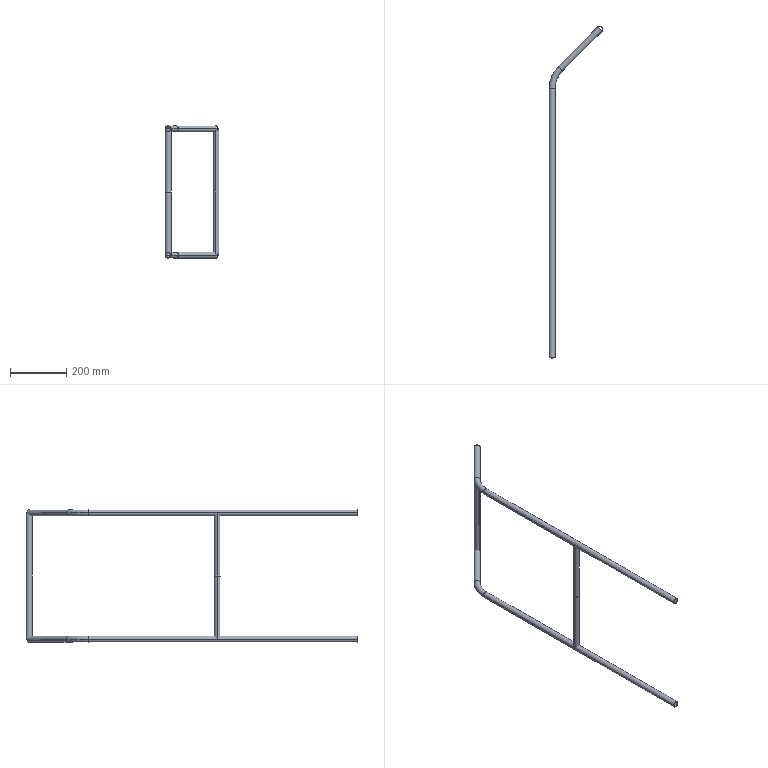Part | SolidWorks | features WeldMemberFeat 3, MirrorSolid 1, WeldmentFeature 1 | 9 solids | 54 faces | box 192.011 x 1181 x 471.3 mm | volume 463241 mm3 | cylinder 28 | plane 18 | torus 8 | commonest cylinder face diameters 16.7 x14 21.3 x14
STEP:
#1=CARTESIAN_POINT('',(-10.65,458.579,0.));
#2=VERTEX_POINT('',#1);
#3=CARTESIAN_POINT('',(10.65,458.579,0.));
#4=VERTEX_POINT('',#3);
#5=CARTESIAN_POINT('',(0.,458.579,0.));
#6=DIRECTION('',(0.,1.,0.));
#7=DIRECTION('',(-1.,0.,0.));
#8=AXIS2_PLACEMENT_3D('',#5,#6,#7);
#9=CIRCLE('',#8,10.65);
#10=EDGE_CURVE('',#2,#4,#9,.T.);
#11=ORIENTED_EDGE('',*,*,#10,.F.);
#12=CARTESIAN_POINT('',(-10.65,-500.,0.));
#13=VERTEX_POINT('',#12);
#14=CARTESIAN_POINT('',(-10.65,458.579,0.));
#15=DIRECTION('',(0.,-1.,0.));
#16=VECTOR('',#15,1000.);
#17=LINE('',#14,#16);
#18=EDGE_CURVE('',#2,#13,#17,.T.);
#19=ORIENTED_EDGE('',*,*,#18,.T.);
#20=CARTESIAN_POINT('',(10.65,-500.,0.));
#21=VERTEX_POINT('',#20);
#22=CARTESIAN_POINT('',(0.,-500.,0.));
#23=DIRECTION('',(0.,1.,0.));
#24=DIRECTION('',(-1.,0.,0.));
#25=AXIS2_PLACEMENT_3D('',#22,#23,#24);
#26=CIRCLE('',#25,10.65);
#27=EDGE_CURVE('',#13,#21,#26,.T.);
#28=ORIENTED_EDGE('',*,*,#27,.T.);
#29=CARTESIAN_POINT('',(10.65,458.579,0.));
#30=DIRECTION('',(0.,-1.,0.));
#31=VECTOR('',#30,1000.);
#32=LINE('',#29,#31);
#33=EDGE_CURVE('',#4,#21,#32,.T.);
#34=ORIENTED_EDGE('',*,*,#33,.F.);
#35=EDGE_LOOP('',(#11,#19,#28,#34));
#36=FACE_OUTER_BOUND('',#35,.T.);
#37=CARTESIAN_POINT('',(0.,458.579,0.));
#38=DIRECTION('',(0.,-1.,0.));
#39=DIRECTION('',(1.,0.,0.));
#40=AXIS2_PLACEMENT_3D('',#37,#38,#39);
#41=CYLINDRICAL_SURFACE('',#40,10.65);
#42=ADVANCED_FACE('',(#36),#41,.T.);
#43=CARTESIAN_POINT('',(8.35,458.579,0.));
#44=VERTEX_POINT('',#43);
#45=CARTESIAN_POINT('',(-8.35,458.579,0.));
#46=VERTEX_POINT('',#45);
#47=CARTESIAN_POINT('',(0.,458.579,0.));
#48=DIRECTION('',(0.,1.,0.));
#49=DIRECTION('',(-1.,0.,0.));
#50=AXIS2_PLACEMENT_3D('',#47,#48,#49);
#51=CIRCLE('',#50,8.35);
#52=EDGE_CURVE('',#44,#46,#51,.T.);
#53=ORIENTED_EDGE('',*,*,#52,.T.);
#54=CARTESIAN_POINT('',(-8.35,-500.,0.));
#55=VERTEX_POINT('',#54);
#56=CARTESIAN_POINT('',(-8.35,458.579,0.));
#57=DIRECTION('',(0.,-1.,0.));
#58=VECTOR('',#57,1000.);
#59=LINE('',#56,#58);
#60=EDGE_CURVE('',#46,#55,#59,.T.);
#61=ORIENTED_EDGE('',*,*,#60,.T.);
#62=CARTESIAN_POINT('',(8.35,-500.,0.));
#63=VERTEX_POINT('',#62);
#64=CARTESIAN_POINT('',(0.,-500.,0.));
#65=DIRECTION('',(0.,1.,0.));
#66=DIRECTION('',(-1.,0.,0.));
#67=AXIS2_PLACEMENT_3D('',#64,#65,#66);
#68=CIRCLE('',#67,8.35);
#69=EDGE_CURVE('',#63,#55,#68,.T.);
#70=ORIENTED_EDGE('',*,*,#69,.F.);
#71=CARTESIAN_POINT('',(8.35,458.579,0.));
#72=DIRECTION('',(0.,-1.,0.));
#73=VECTOR('',#72,1000.);
#74=LINE('',#71,#73);
#75=EDGE_CURVE('',#44,#63,#74,.T.);
#76=ORIENTED_EDGE('',*,*,#75,.F.);
#77=EDGE_LOOP('',(#53,#61,#70,#76));
#78=FACE_OUTER_BOUND('',#77,.T.);
#79=CARTESIAN_POINT('',(0.,458.579,0.));
#80=DIRECTION('',(0.,-1.,0.));
#81=DIRECTION('',(1.,0.,0.));
#82=AXIS2_PLACEMENT_3D('',#79,#80,#81);
#83=CYLINDRICAL_SURFACE('',#82,8.35);
#84=ADVANCED_FACE('',(#78),#83,.F.);
#85=ORIENTED_EDGE('',*,*,#60,.F.);
#86=CARTESIAN_POINT('',(0.,458.579,0.));
#87=DIRECTION('',(0.,1.,0.));
#88=DIRECTION('',(-1.,0.,0.));
#89=AXIS2_PLACEMENT_3D('',#86,#87,#88);
#90=CIRCLE('',#89,8.35);
#91=EDGE_CURVE('',#46,#44,#90,.T.);
#92=ORIENTED_EDGE('',*,*,#91,.T.);
#93=ORIENTED_EDGE('',*,*,#75,.T.);
#94=CARTESIAN_POINT('',(0.,-500.,0.));
#95=DIRECTION('',(0.,1.,0.));
#96=DIRECTION('',(-1.,0.,0.));
#97=AXIS2_PLACEMENT_3D('',#94,#95,#96);
#98=CIRCLE('',#97,8.35);
#99=EDGE_CURVE('',#55,#63,#98,.T.);
#100=ORIENTED_EDGE('',*,*,#99,.F.);
#101=EDGE_LOOP('',(#85,#92,#93,#100));
#102=FACE_OUTER_BOUND('',#101,.T.);
#103=CARTESIAN_POINT('',(0.,458.579,0.));
#104=DIRECTION('',(0.,-1.,0.));
#105=DIRECTION('',(1.,0.,0.));
#106=AXIS2_PLACEMENT_3D('',#103,#104,#105);
#107=CYLINDRICAL_SURFACE('',#106,8.35);
#108=ADVANCED_FACE('',(#102),#107,.F.);
#109=ORIENTED_EDGE('',*,*,#18,.F.);
#110=CARTESIAN_POINT('',(0.,458.579,0.));
#111=DIRECTION('',(0.,1.,0.));
#112=DIRECTION('',(-1.,0.,0.));
#113=AXIS2_PLACEMENT_3D('',#110,#111,#112);
#114=CIRCLE('',#113,10.65);
#115=EDGE_CURVE('',#4,#2,#114,.T.);
#116=ORIENTED_EDGE('',*,*,#115,.F.);
#117=ORIENTED_EDGE('',*,*,#33,.T.);
#118=CARTESIAN_POINT('',(0.,-500.,0.));
#119=DIRECTION('',(0.,1.,0.));
#120=DIRECTION('',(-1.,0.,0.));
#121=AXIS2_PLACEMENT_3D('',#118,#119,#120);
#122=CIRCLE('',#121,10.65);
#123=EDGE_CURVE('',#21,#13,#122,.T.);
#124=ORIENTED_EDGE('',*,*,#123,.T.);
#125=EDGE_LOOP('',(#109,#116,#117,#124));
#126=FACE_OUTER_BOUND('',#125,.T.);
#127=CARTESIAN_POINT('',(0.,458.579,0.));
#128=DIRECTION('',(0.,-1.,0.));
#129=DIRECTION('',(1.,0.,0.));
#130=AXIS2_PLACEMENT_3D('',#127,#128,#129);
#131=CYLINDRICAL_SURFACE('',#130,10.65);
#132=ADVANCED_FACE('',(#126),#131,.T.);
#133=ORIENTED_EDGE('',*,*,#69,.T.);
#134=ORIENTED_EDGE('',*,*,#99,.T.);
#135=EDGE_LOOP('',(#133,#134));
#136=FACE_BOUND('',#135,.T.);
#137=ORIENTED_EDGE('',*,*,#123,.F.);
#138=ORIENTED_EDGE('',*,*,#27,.F.);
#139=EDGE_LOOP('',(#137,#138));
#140=FACE_OUTER_BOUND('',#139,.T.);
#141=CARTESIAN_POINT('',(0.,-500.,0.));
#142=DIRECTION('',(0.,1.,0.));
#143=DIRECTION('',(-1.,0.,0.));
#144=AXIS2_PLACEMENT_3D('',#141,#142,#143);
#145=PLANE('',#144);
#146=ADVANCED_FACE('',(#136,#140),#145,.F.);
#147=ORIENTED_EDGE('',*,*,#52,.F.);
#148=ORIENTED_EDGE('',*,*,#91,.F.);
#149=EDGE_LOOP('',(#147,#148));
#150=FACE_BOUND('',#149,.T.);
#151=ORIENTED_EDGE('',*,*,#115,.T.);
#152=ORIENTED_EDGE('',*,*,#10,.T.);
#153=EDGE_LOOP('',(#151,#152));
#154=FACE_OUTER_BOUND('',#153,.T.);
#155=CARTESIAN_POINT('',(0.,458.579,0.));
#156=DIRECTION('',(0.,1.,0.));
#157=DIRECTION('',(-1.,0.,0.));
#158=AXIS2_PLACEMENT_3D('',#155,#156,#157);
#159=PLANE('',#158);
#160=ADVANCED_FACE('',(#150,#154),#159,.T.);
#161=CLOSED_SHELL('',(#42,#84,#108,#132,#146,#160));
#162=MANIFOLD_SOLID_BREP('',#161);
#163=CARTESIAN_POINT('',(21.759,536.82,0.));
#164=VERTEX_POINT('',#163);
#165=CARTESIAN_POINT('',(36.82,521.759,0.));
#166=VERTEX_POINT('',#165);
#167=CARTESIAN_POINT('',(29.289,529.289,0.));
#168=DIRECTION('',(0.7071,0.7071,0.));
#169=DIRECTION('',(-0.7071,0.7071,0.));
#170=AXIS2_PLACEMENT_3D('',#167,#168,#169);
#171=CIRCLE('',#170,10.65);
#172=EDGE_CURVE('',#164,#166,#171,.T.);
#173=ORIENTED_EDGE('',*,*,#172,.F.);
#174=CARTESIAN_POINT('',(-10.65,458.579,0.));
#175=VERTEX_POINT('',#174);
#176=CARTESIAN_POINT('',(100.,458.579,0.));
#177=DIRECTION('',(0.,0.,1.));
#178=DIRECTION('',(1.,0.,0.));
#179=AXIS2_PLACEMENT_3D('',#176,#177,#178);
#180=CIRCLE('',#179,110.65);
#181=EDGE_CURVE('',#164,#175,#180,.T.);
#182=ORIENTED_EDGE('',*,*,#181,.T.);
#183=CARTESIAN_POINT('',(10.65,458.579,0.));
#184=VERTEX_POINT('',#183);
#185=CARTESIAN_POINT('',(0.,458.579,0.));
#186=DIRECTION('',(0.,-1.,0.));
#187=DIRECTION('',(1.,0.,0.));
#188=AXIS2_PLACEMENT_3D('',#185,#186,#187);
#189=CIRCLE('',#188,10.65);
#190=EDGE_CURVE('',#184,#175,#189,.T.);
#191=ORIENTED_EDGE('',*,*,#190,.F.);
#192=CARTESIAN_POINT('',(100.,458.579,0.));
#193=DIRECTION('',(0.,0.,1.));
#194=DIRECTION('',(1.,0.,0.));
#195=AXIS2_PLACEMENT_3D('',#192,#193,#194);
#196=CIRCLE('',#195,89.35);
#197=EDGE_CURVE('',#166,#184,#196,.T.);
#198=ORIENTED_EDGE('',*,*,#197,.F.);
#199=EDGE_LOOP('',(#173,#182,#191,#198));
#200=FACE_OUTER_BOUND('',#199,.T.);
#201=CARTESIAN_POINT('',(100.,458.579,0.));
#202=DIRECTION('',(0.,0.,1.));
#203=DIRECTION('',(1.,0.,0.));
#204=AXIS2_PLACEMENT_3D('',#201,#202,#203);
#205=TOROIDAL_SURFACE('',#204,100.,10.65);
#206=ADVANCED_FACE('',(#200),#205,.T.);
#207=CARTESIAN_POINT('',(35.194,523.385,0.));
#208=VERTEX_POINT('',#207);
#209=CARTESIAN_POINT('',(23.385,535.194,0.));
#210=VERTEX_POINT('',#209);
#211=CARTESIAN_POINT('',(29.289,529.289,0.));
#212=DIRECTION('',(0.7071,0.7071,0.));
#213=DIRECTION('',(-0.7071,0.7071,0.));
#214=AXIS2_PLACEMENT_3D('',#211,#212,#213);
#215=CIRCLE('',#214,8.35);
#216=EDGE_CURVE('',#208,#210,#215,.T.);
#217=ORIENTED_EDGE('',*,*,#216,.T.);
#218=CARTESIAN_POINT('',(-8.35,458.579,0.));
#219=VERTEX_POINT('',#218);
#220=CARTESIAN_POINT('',(100.,458.579,0.));
#221=DIRECTION('',(0.,0.,1.));
#222=DIRECTION('',(1.,0.,0.));
#223=AXIS2_PLACEMENT_3D('',#220,#221,#222);
#224=CIRCLE('',#223,108.35);
#225=EDGE_CURVE('',#210,#219,#224,.T.);
#226=ORIENTED_EDGE('',*,*,#225,.T.);
#227=CARTESIAN_POINT('',(8.35,458.579,0.));
#228=VERTEX_POINT('',#227);
#229=CARTESIAN_POINT('',(0.,458.579,0.));
#230=DIRECTION('',(0.,-1.,0.));
#231=DIRECTION('',(1.,0.,0.));
#232=AXIS2_PLACEMENT_3D('',#229,#230,#231);
#233=CIRCLE('',#232,8.35);
#234=EDGE_CURVE('',#219,#228,#233,.T.);
#235=ORIENTED_EDGE('',*,*,#234,.T.);
#236=CARTESIAN_POINT('',(100.,458.579,0.));
#237=DIRECTION('',(0.,0.,1.));
#238=DIRECTION('',(1.,0.,0.));
#239=AXIS2_PLACEMENT_3D('',#236,#237,#238);
#240=CIRCLE('',#239,91.65);
#241=EDGE_CURVE('',#208,#228,#240,.T.);
#242=ORIENTED_EDGE('',*,*,#241,.F.);
#243=EDGE_LOOP('',(#217,#226,#235,#242));
#244=FACE_OUTER_BOUND('',#243,.T.);
#245=CARTESIAN_POINT('',(100.,458.579,0.));
#246=DIRECTION('',(0.,0.,1.));
#247=DIRECTION('',(1.,0.,0.));
#248=AXIS2_PLACEMENT_3D('',#245,#246,#247);
#249=TOROIDAL_SURFACE('',#248,100.,8.35);
#250=ADVANCED_FACE('',(#244),#249,.F.);
#251=ORIENTED_EDGE('',*,*,#225,.F.);
#252=CARTESIAN_POINT('',(29.289,529.289,0.));
#253=DIRECTION('',(0.7071,0.7071,0.));
#254=DIRECTION('',(-0.7071,0.7071,0.));
#255=AXIS2_PLACEMENT_3D('',#252,#253,#254);
#256=CIRCLE('',#255,8.35);
#257=EDGE_CURVE('',#210,#208,#256,.T.);
#258=ORIENTED_EDGE('',*,*,#257,.T.);
#259=ORIENTED_EDGE('',*,*,#241,.T.);
#260=CARTESIAN_POINT('',(0.,458.579,0.));
#261=DIRECTION('',(0.,-1.,0.));
#262=DIRECTION('',(1.,0.,0.));
#263=AXIS2_PLACEMENT_3D('',#260,#261,#262);
#264=CIRCLE('',#263,8.35);
#265=EDGE_CURVE('',#228,#219,#264,.T.);
#266=ORIENTED_EDGE('',*,*,#265,.T.);
#267=EDGE_LOOP('',(#251,#258,#259,#266));
#268=FACE_OUTER_BOUND('',#267,.T.);
#269=CARTESIAN_POINT('',(100.,458.579,0.));
#270=DIRECTION('',(0.,0.,1.));
#271=DIRECTION('',(1.,0.,0.));
#272=AXIS2_PLACEMENT_3D('',#269,#270,#271);
#273=TOROIDAL_SURFACE('',#272,100.,8.35);
#274=ADVANCED_FACE('',(#268),#273,.F.);
#275=ORIENTED_EDGE('',*,*,#181,.F.);
#276=CARTESIAN_POINT('',(29.289,529.289,0.));
#277=DIRECTION('',(0.7071,0.7071,0.));
#278=DIRECTION('',(-0.7071,0.7071,0.));
#279=AXIS2_PLACEMENT_3D('',#276,#277,#278);
#280=CIRCLE('',#279,10.65);
#281=EDGE_CURVE('',#166,#164,#280,.T.);
#282=ORIENTED_EDGE('',*,*,#281,.F.);
#283=ORIENTED_EDGE('',*,*,#197,.T.);
#284=CARTESIAN_POINT('',(0.,458.579,0.));
#285=DIRECTION('',(0.,-1.,0.));
#286=DIRECTION('',(1.,0.,0.));
#287=AXIS2_PLACEMENT_3D('',#284,#285,#286);
#288=CIRCLE('',#287,10.65);
#289=EDGE_CURVE('',#175,#184,#288,.T.);
#290=ORIENTED_EDGE('',*,*,#289,.F.);
#291=EDGE_LOOP('',(#275,#282,#283,#290));
#292=FACE_OUTER_BOUND('',#291,.T.);
#293=CARTESIAN_POINT('',(100.,458.579,0.));
#294=DIRECTION('',(0.,0.,1.));
#295=DIRECTION('',(1.,0.,0.));
#296=AXIS2_PLACEMENT_3D('',#293,#294,#295);
#297=TOROIDAL_SURFACE('',#296,100.,10.65);
#298=ADVANCED_FACE('',(#292),#297,.T.);
#299=ORIENTED_EDGE('',*,*,#216,.F.);
#300=ORIENTED_EDGE('',*,*,#257,.F.);
#301=EDGE_LOOP('',(#299,#300));
#302=FACE_BOUND('',#301,.T.);
#303=ORIENTED_EDGE('',*,*,#281,.T.);
#304=ORIENTED_EDGE('',*,*,#172,.T.);
#305=EDGE_LOOP('',(#303,#304));
#306=FACE_OUTER_BOUND('',#305,.T.);
#307=CARTESIAN_POINT('',(29.289,529.289,0.));
#308=DIRECTION('',(0.7071,0.7071,0.));
#309=DIRECTION('',(-0.7071,0.7071,0.));
#310=AXIS2_PLACEMENT_3D('',#307,#308,#309);
#311=PLANE('',#310);
#312=ADVANCED_FACE('',(#302,#306),#311,.T.);
#313=ORIENTED_EDGE('',*,*,#265,.F.);
#314=ORIENTED_EDGE('',*,*,#234,.F.);
#315=EDGE_LOOP('',(#313,#314));
#316=FACE_BOUND('',#315,.T.);
#317=ORIENTED_EDGE('',*,*,#190,.T.);
#318=ORIENTED_EDGE('',*,*,#289,.T.);
#319=EDGE_LOOP('',(#317,#318));
#320=FACE_OUTER_BOUND('',#319,.T.);
#321=CARTESIAN_POINT('',(0.,458.579,0.));
#322=DIRECTION('',(0.,-1.,0.));
#323=DIRECTION('',(1.,0.,0.));
#324=AXIS2_PLACEMENT_3D('',#321,#322,#323);
#325=PLANE('',#324);
#326=ADVANCED_FACE('',(#316,#320),#325,.T.);
#327=CLOSED_SHELL('',(#206,#250,#274,#298,#312,#326));
#328=MANIFOLD_SOLID_BREP('',#327);
#329=CARTESIAN_POINT('',(163.18,678.241,0.));
#330=VERTEX_POINT('',#329);
#331=CARTESIAN_POINT('',(178.241,663.18,0.));
#332=VERTEX_POINT('',#331);
#333=CARTESIAN_POINT('',(170.711,670.711,0.));
#334=DIRECTION('',(0.7071,0.7071,0.));
#335=DIRECTION('',(-0.7071,0.7071,0.));
#336=AXIS2_PLACEMENT_3D('',#333,#334,#335);
#337=CIRCLE('',#336,10.65);
#338=EDGE_CURVE('',#330,#332,#337,.T.);
#339=ORIENTED_EDGE('',*,*,#338,.F.);
#340=CARTESIAN_POINT('',(21.759,536.82,0.));
#341=VERTEX_POINT('',#340);
#342=CARTESIAN_POINT('',(163.18,678.241,0.));
#343=DIRECTION('',(-0.7071,-0.7071,0.));
#344=VECTOR('',#343,1000.);
#345=LINE('',#342,#344);
#346=EDGE_CURVE('',#330,#341,#345,.T.);
#347=ORIENTED_EDGE('',*,*,#346,.T.);
#348=CARTESIAN_POINT('',(36.82,521.759,0.));
#349=VERTEX_POINT('',#348);
#350=CARTESIAN_POINT('',(29.289,529.289,0.));
#351=DIRECTION('',(-0.7071,-0.7071,0.));
#352=DIRECTION('',(0.7071,-0.7071,0.));
#353=AXIS2_PLACEMENT_3D('',#350,#351,#352);
#354=CIRCLE('',#353,10.65);
#355=EDGE_CURVE('',#349,#341,#354,.T.);
#356=ORIENTED_EDGE('',*,*,#355,.F.);
#357=CARTESIAN_POINT('',(178.241,663.18,0.));
#358=DIRECTION('',(-0.7071,-0.7071,0.));
#359=VECTOR('',#358,1000.);
#360=LINE('',#357,#359);
#361=EDGE_CURVE('',#332,#349,#360,.T.);
#362=ORIENTED_EDGE('',*,*,#361,.F.);
#363=EDGE_LOOP('',(#339,#347,#356,#362));
#364=FACE_OUTER_BOUND('',#363,.T.);
#365=CARTESIAN_POINT('',(170.711,670.711,0.));
#366=DIRECTION('',(-0.7071,-0.7071,0.));
#367=DIRECTION('',(0.7071,-0.7071,0.));
#368=AXIS2_PLACEMENT_3D('',#365,#366,#367);
#369=CYLINDRICAL_SURFACE('',#368,10.65);
#370=ADVANCED_FACE('',(#364),#369,.T.);
#371=CARTESIAN_POINT('',(176.615,664.806,0.));
#372=VERTEX_POINT('',#371);
#373=CARTESIAN_POINT('',(164.806,676.615,0.));
#374=VERTEX_POINT('',#373);
#375=CARTESIAN_POINT('',(170.711,670.711,0.));
#376=DIRECTION('',(0.7071,0.7071,0.));
#377=DIRECTION('',(-0.7071,0.7071,0.));
#378=AXIS2_PLACEMENT_3D('',#375,#376,#377);
#379=CIRCLE('',#378,8.35);
#380=EDGE_CURVE('',#372,#374,#379,.T.);
#381=ORIENTED_EDGE('',*,*,#380,.T.);
#382=CARTESIAN_POINT('',(23.385,535.194,0.));
#383=VERTEX_POINT('',#382);
#384=CARTESIAN_POINT('',(164.806,676.615,0.));
#385=DIRECTION('',(-0.7071,-0.7071,0.));
#386=VECTOR('',#385,1000.);
#387=LINE('',#384,#386);
#388=EDGE_CURVE('',#374,#383,#387,.T.);
#389=ORIENTED_EDGE('',*,*,#388,.T.);
#390=CARTESIAN_POINT('',(35.194,523.385,0.));
#391=VERTEX_POINT('',#390);
#392=CARTESIAN_POINT('',(29.289,529.289,0.));
#393=DIRECTION('',(-0.7071,-0.7071,0.));
#394=DIRECTION('',(0.7071,-0.7071,0.));
#395=AXIS2_PLACEMENT_3D('',#392,#393,#394);
#396=CIRCLE('',#395,8.35);
#397=EDGE_CURVE('',#383,#391,#396,.T.);
#398=ORIENTED_EDGE('',*,*,#397,.T.);
#399=CARTESIAN_POINT('',(176.615,664.806,0.));
#400=DIRECTION('',(-0.7071,-0.7071,0.));
#401=VECTOR('',#400,1000.);
#402=LINE('',#399,#401);
#403=EDGE_CURVE('',#372,#391,#402,.T.);
#404=ORIENTED_EDGE('',*,*,#403,.F.);
#405=EDGE_LOOP('',(#381,#389,#398,#404));
#406=FACE_OUTER_BOUND('',#405,.T.);
#407=CARTESIAN_POINT('',(170.711,670.711,0.));
#408=DIRECTION('',(-0.7071,-0.7071,0.));
#409=DIRECTION('',(0.7071,-0.7071,0.));
#410=AXIS2_PLACEMENT_3D('',#407,#408,#409);
#411=CYLINDRICAL_SURFACE('',#410,8.35);
#412=ADVANCED_FACE('',(#406),#411,.F.);
#413=ORIENTED_EDGE('',*,*,#388,.F.);
#414=CARTESIAN_POINT('',(170.711,670.711,0.));
#415=DIRECTION('',(0.7071,0.7071,0.));
#416=DIRECTION('',(-0.7071,0.7071,0.));
#417=AXIS2_PLACEMENT_3D('',#414,#415,#416);
#418=CIRCLE('',#417,8.35);
#419=EDGE_CURVE('',#374,#372,#418,.T.);
#420=ORIENTED_EDGE('',*,*,#419,.T.);
#421=ORIENTED_EDGE('',*,*,#403,.T.);
#422=CARTESIAN_POINT('',(29.289,529.289,0.));
#423=DIRECTION('',(-0.7071,-0.7071,0.));
#424=DIRECTION('',(0.7071,-0.7071,0.));
#425=AXIS2_PLACEMENT_3D('',#422,#423,#424);
#426=CIRCLE('',#425,8.35);
#427=EDGE_CURVE('',#391,#383,#426,.T.);
#428=ORIENTED_EDGE('',*,*,#427,.T.);
#429=EDGE_LOOP('',(#413,#420,#421,#428));
#430=FACE_OUTER_BOUND('',#429,.T.);
#431=CARTESIAN_POINT('',(170.711,670.711,0.));
#432=DIRECTION('',(-0.7071,-0.7071,0.));
#433=DIRECTION('',(0.7071,-0.7071,0.));
#434=AXIS2_PLACEMENT_3D('',#431,#432,#433);
#435=CYLINDRICAL_SURFACE('',#434,8.35);
#436=ADVANCED_FACE('',(#430),#435,.F.);
#437=ORIENTED_EDGE('',*,*,#346,.F.);
#438=CARTESIAN_POINT('',(170.711,670.711,0.));
#439=DIRECTION('',(0.7071,0.7071,0.));
#440=DIRECTION('',(-0.7071,0.7071,0.));
#441=AXIS2_PLACEMENT_3D('',#438,#439,#440);
#442=CIRCLE('',#441,10.65);
#443=EDGE_CURVE('',#332,#330,#442,.T.);
#444=ORIENTED_EDGE('',*,*,#443,.F.);
#445=ORIENTED_EDGE('',*,*,#361,.T.);
#446=CARTESIAN_POINT('',(29.289,529.289,0.));
#447=DIRECTION('',(-0.7071,-0.7071,0.));
#448=DIRECTION('',(0.7071,-0.7071,0.));
#449=AXIS2_PLACEMENT_3D('',#446,#447,#448);
#450=CIRCLE('',#449,10.65);
#451=EDGE_CURVE('',#341,#349,#450,.T.);
#452=ORIENTED_EDGE('',*,*,#451,.F.);
#453=EDGE_LOOP('',(#437,#444,#445,#452));
#454=FACE_OUTER_BOUND('',#453,.T.);
#455=CARTESIAN_POINT('',(170.711,670.711,0.));
#456=DIRECTION('',(-0.7071,-0.7071,0.));
#457=DIRECTION('',(0.7071,-0.7071,0.));
#458=AXIS2_PLACEMENT_3D('',#455,#456,#457);
#459=CYLINDRICAL_SURFACE('',#458,10.65);
#460=ADVANCED_FACE('',(#454),#459,.T.);
#461=ORIENTED_EDGE('',*,*,#380,.F.);
#462=ORIENTED_EDGE('',*,*,#419,.F.);
#463=EDGE_LOOP('',(#461,#462));
#464=FACE_BOUND('',#463,.T.);
#465=ORIENTED_EDGE('',*,*,#443,.T.);
#466=ORIENTED_EDGE('',*,*,#338,.T.);
#467=EDGE_LOOP('',(#465,#466));
#468=FACE_OUTER_BOUND('',#467,.T.);
#469=CARTESIAN_POINT('',(170.711,670.711,0.));
#470=DIRECTION('',(0.7071,0.7071,0.));
#471=DIRECTION('',(-0.7071,0.7071,0.));
#472=AXIS2_PLACEMENT_3D('',#469,#470,#471);
#473=PLANE('',#472);
#474=ADVANCED_FACE('',(#464,#468),#473,.T.);
#475=ORIENTED_EDGE('',*,*,#427,.F.);
#476=ORIENTED_EDGE('',*,*,#397,.F.);
#477=EDGE_LOOP('',(#475,#476));
#478=FACE_BOUND('',#477,.T.);
#479=ORIENTED_EDGE('',*,*,#355,.T.);
#480=ORIENTED_EDGE('',*,*,#451,.T.);
#481=EDGE_LOOP('',(#479,#480));
#482=FACE_OUTER_BOUND('',#481,.T.);
#483=CARTESIAN_POINT('',(29.289,529.289,0.));
#484=DIRECTION('',(-0.7071,-0.7071,0.));
#485=DIRECTION('',(0.7071,-0.7071,0.));
#486=AXIS2_PLACEMENT_3D('',#483,#484,#485);
#487=PLANE('',#486);
#488=ADVANCED_FACE('',(#478,#482),#487,.T.);
#489=CLOSED_SHELL('',(#370,#412,#436,#460,#474,#488));
#490=MANIFOLD_SOLID_BREP('',#489);
#491=CARTESIAN_POINT('',(10.65,0.,225.));
#492=VERTEX_POINT('',#491);
#493=CARTESIAN_POINT('',(-10.65,0.,225.));
#494=VERTEX_POINT('',#493);
#495=CARTESIAN_POINT('',(0.,0.,225.));
#496=DIRECTION('',(0.,0.,1.));
#497=DIRECTION('',(1.,0.,0.));
#498=AXIS2_PLACEMENT_3D('',#495,#496,#497);
#499=CIRCLE('',#498,10.65);
#500=EDGE_CURVE('',#492,#494,#499,.T.);
#501=ORIENTED_EDGE('',*,*,#500,.F.);
#502=CARTESIAN_POINT('',(10.65,0.,0.));
#503=VERTEX_POINT('',#502);
#504=CARTESIAN_POINT('',(10.65,0.,225.));
#505=DIRECTION('',(0.,0.,-1.));
#506=VECTOR('',#505,1000.);
#507=LINE('',#504,#506);
#508=EDGE_CURVE('',#492,#503,#507,.T.);
#509=ORIENTED_EDGE('',*,*,#508,.T.);
#510=CARTESIAN_POINT('',(-10.65,0.,0.));
#511=VERTEX_POINT('',#510);
#512=CARTESIAN_POINT('',(0.,0.,0.));
#513=DIRECTION('',(0.,0.,1.));
#514=DIRECTION('',(1.,0.,0.));
#515=AXIS2_PLACEMENT_3D('',#512,#513,#514);
#516=CIRCLE('',#515,10.65);
#517=EDGE_CURVE('',#503,#511,#516,.T.);
#518=ORIENTED_EDGE('',*,*,#517,.T.);
#519=CARTESIAN_POINT('',(-10.65,0.,225.));
#520=DIRECTION('',(0.,0.,-1.));
#521=VECTOR('',#520,1000.);
#522=LINE('',#519,#521);
#523=EDGE_CURVE('',#494,#511,#522,.T.);
#524=ORIENTED_EDGE('',*,*,#523,.F.);
#525=EDGE_LOOP('',(#501,#509,#518,#524));
#526=FACE_OUTER_BOUND('',#525,.T.);
#527=CARTESIAN_POINT('',(0.,0.,225.));
#528=DIRECTION('',(0.,0.,-1.));
#529=DIRECTION('',(-1.,0.,0.));
#530=AXIS2_PLACEMENT_3D('',#527,#528,#529);
#531=CYLINDRICAL_SURFACE('',#530,10.65);
#532=ADVANCED_FACE('',(#526),#531,.T.);
#533=CARTESIAN_POINT('',(-8.35,0.,225.));
#534=VERTEX_POINT('',#533);
#535=CARTESIAN_POINT('',(8.35,0.,225.));
#536=VERTEX_POINT('',#535);
#537=CARTESIAN_POINT('',(0.,0.,225.));
#538=DIRECTION('',(0.,0.,1.));
#539=DIRECTION('',(1.,0.,0.));
#540=AXIS2_PLACEMENT_3D('',#537,#538,#539);
#541=CIRCLE('',#540,8.35);
#542=EDGE_CURVE('',#534,#536,#541,.T.);
#543=ORIENTED_EDGE('',*,*,#542,.T.);
#544=CARTESIAN_POINT('',(8.35,0.,0.));
#545=VERTEX_POINT('',#544);
#546=CARTESIAN_POINT('',(8.35,0.,225.));
#547=DIRECTION('',(0.,0.,-1.));
#548=VECTOR('',#547,1000.);
#549=LINE('',#546,#548);
#550=EDGE_CURVE('',#536,#545,#549,.T.);
#551=ORIENTED_EDGE('',*,*,#550,.T.);
#552=CARTESIAN_POINT('',(-8.35,0.,0.));
#553=VERTEX_POINT('',#552);
#554=CARTESIAN_POINT('',(0.,0.,0.));
#555=DIRECTION('',(0.,0.,1.));
#556=DIRECTION('',(1.,0.,0.));
#557=AXIS2_PLACEMENT_3D('',#554,#555,#556);
#558=CIRCLE('',#557,8.35);
#559=EDGE_CURVE('',#553,#545,#558,.T.);
#560=ORIENTED_EDGE('',*,*,#559,.F.);
#561=CARTESIAN_POINT('',(-8.35,0.,225.));
#562=DIRECTION('',(0.,0.,-1.));
#563=VECTOR('',#562,1000.);
#564=LINE('',#561,#563);
#565=EDGE_CURVE('',#534,#553,#564,.T.);
#566=ORIENTED_EDGE('',*,*,#565,.F.);
#567=EDGE_LOOP('',(#543,#551,#560,#566));
#568=FACE_OUTER_BOUND('',#567,.T.);
#569=CARTESIAN_POINT('',(0.,0.,225.));
#570=DIRECTION('',(0.,0.,-1.));
#571=DIRECTION('',(-1.,0.,0.));
#572=AXIS2_PLACEMENT_3D('',#569,#570,#571);
#573=CYLINDRICAL_SURFACE('',#572,8.35);
#574=ADVANCED_FACE('',(#568),#573,.F.);
#575=ORIENTED_EDGE('',*,*,#550,.F.);
#576=CARTESIAN_POINT('',(0.,0.,225.));
#577=DIRECTION('',(0.,0.,1.));
#578=DIRECTION('',(1.,0.,0.));
#579=AXIS2_PLACEMENT_3D('',#576,#577,#578);
#580=CIRCLE('',#579,8.35);
#581=EDGE_CURVE('',#536,#534,#580,.T.);
#582=ORIENTED_EDGE('',*,*,#581,.T.);
#583=ORIENTED_EDGE('',*,*,#565,.T.);
#584=CARTESIAN_POINT('',(0.,0.,0.));
#585=DIRECTION('',(0.,0.,1.));
#586=DIRECTION('',(1.,0.,0.));
#587=AXIS2_PLACEMENT_3D('',#584,#585,#586);
#588=CIRCLE('',#587,8.35);
#589=EDGE_CURVE('',#545,#553,#588,.T.);
#590=ORIENTED_EDGE('',*,*,#589,.F.);
#591=EDGE_LOOP('',(#575,#582,#583,#590));
#592=FACE_OUTER_BOUND('',#591,.T.);
#593=CARTESIAN_POINT('',(0.,0.,225.));
#594=DIRECTION('',(0.,0.,-1.));
#595=DIRECTION('',(-1.,0.,0.));
#596=AXIS2_PLACEMENT_3D('',#593,#594,#595);
#597=CYLINDRICAL_SURFACE('',#596,8.35);
#598=ADVANCED_FACE('',(#592),#597,.F.);
#599=ORIENTED_EDGE('',*,*,#508,.F.);
#600=CARTESIAN_POINT('',(0.,0.,225.));
#601=DIRECTION('',(0.,0.,1.));
#602=DIRECTION('',(1.,0.,0.));
#603=AXIS2_PLACEMENT_3D('',#600,#601,#602);
#604=CIRCLE('',#603,10.65);
#605=EDGE_CURVE('',#494,#492,#604,.T.);
#606=ORIENTED_EDGE('',*,*,#605,.F.);
#607=ORIENTED_EDGE('',*,*,#523,.T.);
#608=CARTESIAN_POINT('',(0.,0.,0.));
#609=DIRECTION('',(0.,0.,1.));
#610=DIRECTION('',(1.,0.,0.));
#611=AXIS2_PLACEMENT_3D('',#608,#609,#610);
#612=CIRCLE('',#611,10.65);
#613=EDGE_CURVE('',#511,#503,#612,.T.);
#614=ORIENTED_EDGE('',*,*,#613,.T.);
#615=EDGE_LOOP('',(#599,#606,#607,#614));
#616=FACE_OUTER_BOUND('',#615,.T.);
#617=CARTESIAN_POINT('',(0.,0.,225.));
#618=DIRECTION('',(0.,0.,-1.));
#619=DIRECTION('',(-1.,0.,0.));
#620=AXIS2_PLACEMENT_3D('',#617,#618,#619);
#621=CYLINDRICAL_SURFACE('',#620,10.65);
#622=ADVANCED_FACE('',(#616),#621,.T.);
#623=ORIENTED_EDGE('',*,*,#542,.F.);
#624=ORIENTED_EDGE('',*,*,#581,.F.);
#625=EDGE_LOOP('',(#623,#624));
#626=FACE_BOUND('',#625,.T.);
#627=ORIENTED_EDGE('',*,*,#605,.T.);
#628=ORIENTED_EDGE('',*,*,#500,.T.);
#629=EDGE_LOOP('',(#627,#628));
#630=FACE_OUTER_BOUND('',#629,.T.);
#631=CARTESIAN_POINT('',(0.,0.,225.));
#632=DIRECTION('',(0.,0.,1.));
#633=DIRECTION('',(1.,0.,0.));
#634=AXIS2_PLACEMENT_3D('',#631,#632,#633);
#635=PLANE('',#634);
#636=ADVANCED_FACE('',(#626,#630),#635,.T.);
#637=ORIENTED_EDGE('',*,*,#559,.T.);
#638=ORIENTED_EDGE('',*,*,#589,.T.);
#639=EDGE_LOOP('',(#637,#638));
#640=FACE_BOUND('',#639,.T.);
#641=ORIENTED_EDGE('',*,*,#613,.F.);
#642=ORIENTED_EDGE('',*,*,#517,.F.);
#643=EDGE_LOOP('',(#641,#642));
#644=FACE_OUTER_BOUND('',#643,.T.);
#645=CARTESIAN_POINT('',(0.,0.,0.));
#646=DIRECTION('',(0.,0.,1.));
#647=DIRECTION('',(1.,0.,0.));
#648=AXIS2_PLACEMENT_3D('',#645,#646,#647);
#649=PLANE('',#648);
#650=ADVANCED_FACE('',(#640,#644),#649,.F.);
#651=CLOSED_SHELL('',(#532,#574,#598,#622,#636,#650));
#652=MANIFOLD_SOLID_BREP('',#651);
#653=CARTESIAN_POINT('',(178.241,663.18,450.));
#654=VERTEX_POINT('',#653);
#655=CARTESIAN_POINT('',(163.18,678.241,450.));
#656=VERTEX_POINT('',#655);
#657=CARTESIAN_POINT('',(170.711,670.711,450.));
#658=DIRECTION('',(-0.7071,-0.7071,0.));
#659=DIRECTION('',(-0.7071,0.7071,0.));
#660=AXIS2_PLACEMENT_3D('',#657,#658,#659);
#661=CIRCLE('',#660,10.65);
#662=EDGE_CURVE('',#654,#656,#661,.T.);
#663=ORIENTED_EDGE('',*,*,#662,.T.);
#664=CARTESIAN_POINT('',(21.759,536.82,450.));
#665=VERTEX_POINT('',#664);
#666=CARTESIAN_POINT('',(163.18,678.241,450.));
#667=DIRECTION('',(-0.7071,-0.7071,0.));
#668=VECTOR('',#667,1000.);
#669=LINE('',#666,#668);
#670=EDGE_CURVE('',#656,#665,#669,.T.);
#671=ORIENTED_EDGE('',*,*,#670,.T.);
#672=CARTESIAN_POINT('',(36.82,521.759,450.));
#673=VERTEX_POINT('',#672);
#674=CARTESIAN_POINT('',(29.289,529.289,450.));
#675=DIRECTION('',(0.7071,0.7071,0.));
#676=DIRECTION('',(0.7071,-0.7071,0.));
#677=AXIS2_PLACEMENT_3D('',#674,#675,#676);
#678=CIRCLE('',#677,10.65);
#679=EDGE_CURVE('',#665,#673,#678,.T.);
#680=ORIENTED_EDGE('',*,*,#679,.T.);
#681=CARTESIAN_POINT('',(178.241,663.18,450.));
#682=DIRECTION('',(-0.7071,-0.7071,0.));
#683=VECTOR('',#682,1000.);
#684=LINE('',#681,#683);
#685=EDGE_CURVE('',#654,#673,#684,.T.);
#686=ORIENTED_EDGE('',*,*,#685,.F.);
#687=EDGE_LOOP('',(#663,#671,#680,#686));
#688=FACE_OUTER_BOUND('',#687,.T.);
#689=CARTESIAN_POINT('',(170.711,670.711,450.));
#690=DIRECTION('',(-0.7071,-0.7071,0.));
#691=DIRECTION('',(0.7071,-0.7071,0.));
#692=AXIS2_PLACEMENT_3D('',#689,#690,#691);
#693=CYLINDRICAL_SURFACE('',#692,10.65);
#694=ADVANCED_FACE('',(#688),#693,.T.);
#695=CARTESIAN_POINT('',(164.806,676.615,450.));
#696=VERTEX_POINT('',#695);
#697=CARTESIAN_POINT('',(176.615,664.806,450.));
#698=VERTEX_POINT('',#697);
#699=CARTESIAN_POINT('',(170.711,670.711,450.));
#700=DIRECTION('',(-0.7071,-0.7071,0.));
#701=DIRECTION('',(-0.7071,0.7071,0.));
#702=AXIS2_PLACEMENT_3D('',#699,#700,#701);
#703=CIRCLE('',#702,8.35);
#704=EDGE_CURVE('',#696,#698,#703,.T.);
#705=ORIENTED_EDGE('',*,*,#704,.F.);
#706=CARTESIAN_POINT('',(23.385,535.194,450.));
#707=VERTEX_POINT('',#706);
#708=CARTESIAN_POINT('',(164.806,676.615,450.));
#709=DIRECTION('',(-0.7071,-0.7071,0.));
#710=VECTOR('',#709,1000.);
#711=LINE('',#708,#710);
#712=EDGE_CURVE('',#696,#707,#711,.T.);
#713=ORIENTED_EDGE('',*,*,#712,.T.);
#714=CARTESIAN_POINT('',(35.194,523.385,450.));
#715=VERTEX_POINT('',#714);
#716=CARTESIAN_POINT('',(29.289,529.289,450.));
#717=DIRECTION('',(0.7071,0.7071,0.));
#718=DIRECTION('',(0.7071,-0.7071,0.));
#719=AXIS2_PLACEMENT_3D('',#716,#717,#718);
#720=CIRCLE('',#719,8.35);
#721=EDGE_CURVE('',#715,#707,#720,.T.);
#722=ORIENTED_EDGE('',*,*,#721,.F.);
#723=CARTESIAN_POINT('',(176.615,664.806,450.));
#724=DIRECTION('',(-0.7071,-0.7071,0.));
#725=VECTOR('',#724,1000.);
#726=LINE('',#723,#725);
#727=EDGE_CURVE('',#698,#715,#726,.T.);
#728=ORIENTED_EDGE('',*,*,#727,.F.);
#729=EDGE_LOOP('',(#705,#713,#722,#728));
#730=FACE_OUTER_BOUND('',#729,.T.);
#731=CARTESIAN_POINT('',(170.711,670.711,450.));
#732=DIRECTION('',(-0.7071,-0.7071,0.));
#733=DIRECTION('',(0.7071,-0.7071,0.));
#734=AXIS2_PLACEMENT_3D('',#731,#732,#733);
#735=CYLINDRICAL_SURFACE('',#734,8.35);
#736=ADVANCED_FACE('',(#730),#735,.F.);
#737=ORIENTED_EDGE('',*,*,#712,.F.);
#738=CARTESIAN_POINT('',(170.711,670.711,450.));
#739=DIRECTION('',(-0.7071,-0.7071,0.));
#740=DIRECTION('',(-0.7071,0.7071,0.));
#741=AXIS2_PLACEMENT_3D('',#738,#739,#740);
#742=CIRCLE('',#741,8.35);
#743=EDGE_CURVE('',#698,#696,#742,.T.);
#744=ORIENTED_EDGE('',*,*,#743,.F.);
#745=ORIENTED_EDGE('',*,*,#727,.T.);
#746=CARTESIAN_POINT('',(29.289,529.289,450.));
#747=DIRECTION('',(0.7071,0.7071,0.));
#748=DIRECTION('',(0.7071,-0.7071,0.));
#749=AXIS2_PLACEMENT_3D('',#746,#747,#748);
#750=CIRCLE('',#749,8.35);
#751=EDGE_CURVE('',#707,#715,#750,.T.);
#752=ORIENTED_EDGE('',*,*,#751,.F.);
#753=EDGE_LOOP('',(#737,#744,#745,#752));
#754=FACE_OUTER_BOUND('',#753,.T.);
#755=CARTESIAN_POINT('',(170.711,670.711,450.));
#756=DIRECTION('',(-0.7071,-0.7071,0.));
#757=DIRECTION('',(0.7071,-0.7071,0.));
#758=AXIS2_PLACEMENT_3D('',#755,#756,#757);
#759=CYLINDRICAL_SURFACE('',#758,8.35);
#760=ADVANCED_FACE('',(#754),#759,.F.);
#761=ORIENTED_EDGE('',*,*,#670,.F.);
#762=CARTESIAN_POINT('',(170.711,670.711,450.));
#763=DIRECTION('',(-0.7071,-0.7071,0.));
#764=DIRECTION('',(-0.7071,0.7071,0.));
#765=AXIS2_PLACEMENT_3D('',#762,#763,#764);
#766=CIRCLE('',#765,10.65);
#767=EDGE_CURVE('',#656,#654,#766,.T.);
#768=ORIENTED_EDGE('',*,*,#767,.T.);
#769=ORIENTED_EDGE('',*,*,#685,.T.);
#770=CARTESIAN_POINT('',(29.289,529.289,450.));
#771=DIRECTION('',(0.7071,0.7071,0.));
#772=DIRECTION('',(0.7071,-0.7071,0.));
#773=AXIS2_PLACEMENT_3D('',#770,#771,#772);
#774=CIRCLE('',#773,10.65);
#775=EDGE_CURVE('',#673,#665,#774,.T.);
#776=ORIENTED_EDGE('',*,*,#775,.T.);
#777=EDGE_LOOP('',(#761,#768,#769,#776));
#778=FACE_OUTER_BOUND('',#777,.T.);
#779=CARTESIAN_POINT('',(170.711,670.711,450.));
#780=DIRECTION('',(-0.7071,-0.7071,0.));
#781=DIRECTION('',(0.7071,-0.7071,0.));
#782=AXIS2_PLACEMENT_3D('',#779,#780,#781);
#783=CYLINDRICAL_SURFACE('',#782,10.65);
#784=ADVANCED_FACE('',(#778),#783,.T.);
#785=ORIENTED_EDGE('',*,*,#743,.T.);
#786=ORIENTED_EDGE('',*,*,#704,.T.);
#787=EDGE_LOOP('',(#785,#786));
#788=FACE_BOUND('',#787,.T.);
#789=ORIENTED_EDGE('',*,*,#662,.F.);
#790=ORIENTED_EDGE('',*,*,#767,.F.);
#791=EDGE_LOOP('',(#789,#790));
#792=FACE_OUTER_BOUND('',#791,.T.);
#793=CARTESIAN_POINT('',(170.711,670.711,450.));
#794=DIRECTION('',(0.7071,0.7071,0.));
#795=DIRECTION('',(-0.7071,0.7071,0.));
#796=AXIS2_PLACEMENT_3D('',#793,#794,#795);
#797=PLANE('',#796);
#798=ADVANCED_FACE('',(#788,#792),#797,.T.);
#799=ORIENTED_EDGE('',*,*,#721,.T.);
#800=ORIENTED_EDGE('',*,*,#751,.T.);
#801=EDGE_LOOP('',(#799,#800));
#802=FACE_BOUND('',#801,.T.);
#803=ORIENTED_EDGE('',*,*,#775,.F.);
#804=ORIENTED_EDGE('',*,*,#679,.F.);
#805=EDGE_LOOP('',(#803,#804));
#806=FACE_OUTER_BOUND('',#805,.T.);
#807=CARTESIAN_POINT('',(29.289,529.289,450.));
#808=DIRECTION('',(-0.7071,-0.7071,0.));
#809=DIRECTION('',(0.7071,-0.7071,0.));
#810=AXIS2_PLACEMENT_3D('',#807,#808,#809);
#811=PLANE('',#810);
#812=ADVANCED_FACE('',(#802,#806),#811,.T.);
#813=CLOSED_SHELL('',(#694,#736,#760,#784,#798,#812));
#814=MANIFOLD_SOLID_BREP('',#813);
#815=CARTESIAN_POINT('',(10.65,458.579,450.));
#816=VERTEX_POINT('',#815);
#817=CARTESIAN_POINT('',(-10.65,458.579,450.));
#818=VERTEX_POINT('',#817);
#819=CARTESIAN_POINT('',(0.,458.579,450.));
#820=DIRECTION('',(0.,1.,0.));
#821=DIRECTION('',(1.,0.,0.));
#822=AXIS2_PLACEMENT_3D('',#819,#820,#821);
#823=CIRCLE('',#822,10.65);
#824=EDGE_CURVE('',#816,#818,#823,.T.);
#825=ORIENTED_EDGE('',*,*,#824,.T.);
#826=CARTESIAN_POINT('',(21.759,536.82,450.));
#827=VERTEX_POINT('',#826);
#828=CARTESIAN_POINT('',(100.,458.579,450.));
#829=DIRECTION('',(0.,0.,-1.));
#830=DIRECTION('',(-1.,0.,0.));
#831=AXIS2_PLACEMENT_3D('',#828,#829,#830);
#832=CIRCLE('',#831,110.65);
#833=EDGE_CURVE('',#818,#827,#832,.T.);
#834=ORIENTED_EDGE('',*,*,#833,.T.);
#835=CARTESIAN_POINT('',(36.82,521.759,450.));
#836=VERTEX_POINT('',#835);
#837=CARTESIAN_POINT('',(29.289,529.289,450.));
#838=DIRECTION('',(-0.7071,-0.7071,0.));
#839=DIRECTION('',(-0.7071,0.7071,0.));
#840=AXIS2_PLACEMENT_3D('',#837,#838,#839);
#841=CIRCLE('',#840,10.65);
#842=EDGE_CURVE('',#827,#836,#841,.T.);
#843=ORIENTED_EDGE('',*,*,#842,.T.);
#844=CARTESIAN_POINT('',(100.,458.579,450.));
#845=DIRECTION('',(0.,0.,-1.));
#846=DIRECTION('',(-1.,0.,0.));
#847=AXIS2_PLACEMENT_3D('',#844,#845,#846);
#848=CIRCLE('',#847,89.35);
#849=EDGE_CURVE('',#816,#836,#848,.T.);
#850=ORIENTED_EDGE('',*,*,#849,.F.);
#851=EDGE_LOOP('',(#825,#834,#843,#850));
#852=FACE_OUTER_BOUND('',#851,.T.);
#853=CARTESIAN_POINT('',(100.,458.579,450.));
#854=DIRECTION('',(0.,0.,-1.));
#855=DIRECTION('',(1.,0.,0.));
#856=AXIS2_PLACEMENT_3D('',#853,#854,#855);
#857=TOROIDAL_SURFACE('',#856,100.,10.65);
#858=ADVANCED_FACE('',(#852),#857,.T.);
#859=CARTESIAN_POINT('',(-8.35,458.579,450.));
#860=VERTEX_POINT('',#859);
#861=CARTESIAN_POINT('',(8.35,458.579,450.));
#862=VERTEX_POINT('',#861);
#863=CARTESIAN_POINT('',(0.,458.579,450.));
#864=DIRECTION('',(0.,1.,0.));
#865=DIRECTION('',(1.,0.,0.));
#866=AXIS2_PLACEMENT_3D('',#863,#864,#865);
#867=CIRCLE('',#866,8.35);
#868=EDGE_CURVE('',#860,#862,#867,.T.);
#869=ORIENTED_EDGE('',*,*,#868,.F.);
#870=CARTESIAN_POINT('',(23.385,535.194,450.));
#871=VERTEX_POINT('',#870);
#872=CARTESIAN_POINT('',(100.,458.579,450.));
#873=DIRECTION('',(0.,0.,-1.));
#874=DIRECTION('',(-1.,0.,0.));
#875=AXIS2_PLACEMENT_3D('',#872,#873,#874);
#876=CIRCLE('',#875,108.35);
#877=EDGE_CURVE('',#860,#871,#876,.T.);
#878=ORIENTED_EDGE('',*,*,#877,.T.);
#879=CARTESIAN_POINT('',(35.194,523.385,450.));
#880=VERTEX_POINT('',#879);
#881=CARTESIAN_POINT('',(29.289,529.289,450.));
#882=DIRECTION('',(-0.7071,-0.7071,0.));
#883=DIRECTION('',(-0.7071,0.7071,0.));
#884=AXIS2_PLACEMENT_3D('',#881,#882,#883);
#885=CIRCLE('',#884,8.35);
#886=EDGE_CURVE('',#880,#871,#885,.T.);
#887=ORIENTED_EDGE('',*,*,#886,.F.);
#888=CARTESIAN_POINT('',(100.,458.579,450.));
#889=DIRECTION('',(0.,0.,-1.));
#890=DIRECTION('',(-1.,0.,0.));
#891=AXIS2_PLACEMENT_3D('',#888,#889,#890);
#892=CIRCLE('',#891,91.65);
#893=EDGE_CURVE('',#862,#880,#892,.T.);
#894=ORIENTED_EDGE('',*,*,#893,.F.);
#895=EDGE_LOOP('',(#869,#878,#887,#894));
#896=FACE_OUTER_BOUND('',#895,.T.);
#897=CARTESIAN_POINT('',(100.,458.579,450.));
#898=DIRECTION('',(0.,0.,-1.));
#899=DIRECTION('',(1.,0.,0.));
#900=AXIS2_PLACEMENT_3D('',#897,#898,#899);
#901=TOROIDAL_SURFACE('',#900,100.,8.35);
#902=ADVANCED_FACE('',(#896),#901,.F.);
#903=ORIENTED_EDGE('',*,*,#877,.F.);
#904=CARTESIAN_POINT('',(0.,458.579,450.));
#905=DIRECTION('',(0.,1.,0.));
#906=DIRECTION('',(1.,0.,0.));
#907=AXIS2_PLACEMENT_3D('',#904,#905,#906);
#908=CIRCLE('',#907,8.35);
#909=EDGE_CURVE('',#862,#860,#908,.T.);
#910=ORIENTED_EDGE('',*,*,#909,.F.);
#911=ORIENTED_EDGE('',*,*,#893,.T.);
#912=CARTESIAN_POINT('',(29.289,529.289,450.));
#913=DIRECTION('',(-0.7071,-0.7071,0.));
#914=DIRECTION('',(-0.7071,0.7071,0.));
#915=AXIS2_PLACEMENT_3D('',#912,#913,#914);
#916=CIRCLE('',#915,8.35);
#917=EDGE_CURVE('',#871,#880,#916,.T.);
#918=ORIENTED_EDGE('',*,*,#917,.F.);
#919=EDGE_LOOP('',(#903,#910,#911,#918));
#920=FACE_OUTER_BOUND('',#919,.T.);
#921=CARTESIAN_POINT('',(100.,458.579,450.));
#922=DIRECTION('',(0.,0.,-1.));
#923=DIRECTION('',(1.,0.,0.));
#924=AXIS2_PLACEMENT_3D('',#921,#922,#923);
#925=TOROIDAL_SURFACE('',#924,100.,8.35);
#926=ADVANCED_FACE('',(#920),#925,.F.);
#927=ORIENTED_EDGE('',*,*,#833,.F.);
#928=CARTESIAN_POINT('',(0.,458.579,450.));
#929=DIRECTION('',(0.,1.,0.));
#930=DIRECTION('',(1.,0.,0.));
#931=AXIS2_PLACEMENT_3D('',#928,#929,#930);
#932=CIRCLE('',#931,10.65);
#933=EDGE_CURVE('',#818,#816,#932,.T.);
#934=ORIENTED_EDGE('',*,*,#933,.T.);
#935=ORIENTED_EDGE('',*,*,#849,.T.);
#936=CARTESIAN_POINT('',(29.289,529.289,450.));
#937=DIRECTION('',(-0.7071,-0.7071,0.));
#938=DIRECTION('',(-0.7071,0.7071,0.));
#939=AXIS2_PLACEMENT_3D('',#936,#937,#938);
#940=CIRCLE('',#939,10.65);
#941=EDGE_CURVE('',#836,#827,#940,.T.);
#942=ORIENTED_EDGE('',*,*,#941,.T.);
#943=EDGE_LOOP('',(#927,#934,#935,#942));
#944=FACE_OUTER_BOUND('',#943,.T.);
#945=CARTESIAN_POINT('',(100.,458.579,450.));
#946=DIRECTION('',(0.,0.,-1.));
#947=DIRECTION('',(1.,0.,0.));
#948=AXIS2_PLACEMENT_3D('',#945,#946,#947);
#949=TOROIDAL_SURFACE('',#948,100.,10.65);
#950=ADVANCED_FACE('',(#944),#949,.T.);
#951=ORIENTED_EDGE('',*,*,#886,.T.);
#952=ORIENTED_EDGE('',*,*,#917,.T.);
#953=EDGE_LOOP('',(#951,#952));
#954=FACE_BOUND('',#953,.T.);
#955=ORIENTED_EDGE('',*,*,#941,.F.);
#956=ORIENTED_EDGE('',*,*,#842,.F.);
#957=EDGE_LOOP('',(#955,#956));
#958=FACE_OUTER_BOUND('',#957,.T.);
#959=CARTESIAN_POINT('',(29.289,529.289,450.));
#960=DIRECTION('',(0.7071,0.7071,0.));
#961=DIRECTION('',(-0.7071,0.7071,0.));
#962=AXIS2_PLACEMENT_3D('',#959,#960,#961);
#963=PLANE('',#962);
#964=ADVANCED_FACE('',(#954,#958),#963,.T.);
#965=ORIENTED_EDGE('',*,*,#909,.T.);
#966=ORIENTED_EDGE('',*,*,#868,.T.);
#967=EDGE_LOOP('',(#965,#966));
#968=FACE_BOUND('',#967,.T.);
#969=ORIENTED_EDGE('',*,*,#824,.F.);
#970=ORIENTED_EDGE('',*,*,#933,.F.);
#971=EDGE_LOOP('',(#969,#970));
#972=FACE_OUTER_BOUND('',#971,.T.);
#973=CARTESIAN_POINT('',(0.,458.579,450.));
#974=DIRECTION('',(0.,-1.,0.));
#975=DIRECTION('',(1.,0.,0.));
#976=AXIS2_PLACEMENT_3D('',#973,#974,#975);
#977=PLANE('',#976);
#978=ADVANCED_FACE('',(#968,#972),#977,.T.);
#979=CLOSED_SHELL('',(#858,#902,#926,#950,#964,#978));
#980=MANIFOLD_SOLID_BREP('',#979);
#981=CARTESIAN_POINT('',(10.65,458.579,450.));
#982=VERTEX_POINT('',#981);
#983=CARTESIAN_POINT('',(-10.65,458.579,450.));
#984=VERTEX_POINT('',#983);
#985=CARTESIAN_POINT('',(0.,458.579,450.));
#986=DIRECTION('',(0.,-1.,0.));
#987=DIRECTION('',(-1.,0.,0.));
#988=AXIS2_PLACEMENT_3D('',#985,#986,#987);
#989=CIRCLE('',#988,10.65);
#990=EDGE_CURVE('',#982,#984,#989,.T.);
#991=ORIENTED_EDGE('',*,*,#990,.T.);
#992=CARTESIAN_POINT('',(-10.65,-500.,450.));
#993=VERTEX_POINT('',#992);
#994=CARTESIAN_POINT('',(-10.65,458.579,450.));
#995=DIRECTION('',(0.,-1.,0.));
#996=VECTOR('',#995,1000.);
#997=LINE('',#994,#996);
#998=EDGE_CURVE('',#984,#993,#997,.T.);
#999=ORIENTED_EDGE('',*,*,#998,.T.);
#1000=CARTESIAN_POINT('',(10.65,-500.,450.));
#1001=VERTEX_POINT('',#1000);
#1002=CARTESIAN_POINT('',(0.,-500.,450.));
#1003=DIRECTION('',(0.,-1.,0.));
#1004=DIRECTION('',(-1.,0.,0.));
#1005=AXIS2_PLACEMENT_3D('',#1002,#1003,#1004);
#1006=CIRCLE('',#1005,10.65);
#1007=EDGE_CURVE('',#1001,#993,#1006,.T.);
#1008=ORIENTED_EDGE('',*,*,#1007,.F.);
#1009=CARTESIAN_POINT('',(10.65,458.579,450.));
#1010=DIRECTION('',(0.,-1.,0.));
#1011=VECTOR('',#1010,1000.);
#1012=LINE('',#1009,#1011);
#1013=EDGE_CURVE('',#982,#1001,#1012,.T.);
#1014=ORIENTED_EDGE('',*,*,#1013,.F.);
#1015=EDGE_LOOP('',(#991,#999,#1008,#1014));
#1016=FACE_OUTER_BOUND('',#1015,.T.);
#1017=CARTESIAN_POINT('',(0.,458.579,450.));
#1018=DIRECTION('',(0.,-1.,0.));
#1019=DIRECTION('',(1.,0.,0.));
#1020=AXIS2_PLACEMENT_3D('',#1017,#1018,#1019);
#1021=CYLINDRICAL_SURFACE('',#1020,10.65);
#1022=ADVANCED_FACE('',(#1016),#1021,.T.);
#1023=CARTESIAN_POINT('',(-8.35,458.579,450.));
#1024=VERTEX_POINT('',#1023);
#1025=CARTESIAN_POINT('',(8.35,458.579,450.));
#1026=VERTEX_POINT('',#1025);
#1027=CARTESIAN_POINT('',(0.,458.579,450.));
#1028=DIRECTION('',(0.,-1.,0.));
#1029=DIRECTION('',(-1.,0.,0.));
#1030=AXIS2_PLACEMENT_3D('',#1027,#1028,#1029);
#1031=CIRCLE('',#1030,8.35);
#1032=EDGE_CURVE('',#1024,#1026,#1031,.T.);
#1033=ORIENTED_EDGE('',*,*,#1032,.F.);
#1034=CARTESIAN_POINT('',(-8.35,-500.,450.));
#1035=VERTEX_POINT('',#1034);
#1036=CARTESIAN_POINT('',(-8.35,458.579,450.));
#1037=DIRECTION('',(0.,-1.,0.));
#1038=VECTOR('',#1037,1000.);
#1039=LINE('',#1036,#1038);
#1040=EDGE_CURVE('',#1024,#1035,#1039,.T.);
#1041=ORIENTED_EDGE('',*,*,#1040,.T.);
#1042=CARTESIAN_POINT('',(8.35,-500.,450.));
#1043=VERTEX_POINT('',#1042);
#1044=CARTESIAN_POINT('',(0.,-500.,450.));
#1045=DIRECTION('',(0.,-1.,0.));
#1046=DIRECTION('',(-1.,0.,0.));
#1047=AXIS2_PLACEMENT_3D('',#1044,#1045,#1046);
#1048=CIRCLE('',#1047,8.35);
#1049=EDGE_CURVE('',#1035,#1043,#1048,.T.);
#1050=ORIENTED_EDGE('',*,*,#1049,.T.);
#1051=CARTESIAN_POINT('',(8.35,458.579,450.));
#1052=DIRECTION('',(0.,-1.,0.));
#1053=VECTOR('',#1052,1000.);
#1054=LINE('',#1051,#1053);
#1055=EDGE_CURVE('',#1026,#1043,#1054,.T.);
#1056=ORIENTED_EDGE('',*,*,#1055,.F.);
#1057=EDGE_LOOP('',(#1033,#1041,#1050,#1056));
#1058=FACE_OUTER_BOUND('',#1057,.T.);
#1059=CARTESIAN_POINT('',(0.,458.579,450.));
#1060=DIRECTION('',(0.,-1.,0.));
#1061=DIRECTION('',(1.,0.,0.));
#1062=AXIS2_PLACEMENT_3D('',#1059,#1060,#1061);
#1063=CYLINDRICAL_SURFACE('',#1062,8.35);
#1064=ADVANCED_FACE('',(#1058),#1063,.F.);
#1065=ORIENTED_EDGE('',*,*,#1040,.F.);
#1066=CARTESIAN_POINT('',(0.,458.579,450.));
#1067=DIRECTION('',(0.,-1.,0.));
#1068=DIRECTION('',(-1.,0.,0.));
#1069=AXIS2_PLACEMENT_3D('',#1066,#1067,#1068);
#1070=CIRCLE('',#1069,8.35);
#1071=EDGE_CURVE('',#1026,#1024,#1070,.T.);
#1072=ORIENTED_EDGE('',*,*,#1071,.F.);
#1073=ORIENTED_EDGE('',*,*,#1055,.T.);
#1074=CARTESIAN_POINT('',(0.,-500.,450.));
#1075=DIRECTION('',(0.,-1.,0.));
#1076=DIRECTION('',(-1.,0.,0.));
#1077=AXIS2_PLACEMENT_3D('',#1074,#1075,#1076);
#1078=CIRCLE('',#1077,8.35);
#1079=EDGE_CURVE('',#1043,#1035,#1078,.T.);
#1080=ORIENTED_EDGE('',*,*,#1079,.T.);
#1081=EDGE_LOOP('',(#1065,#1072,#1073,#1080));
#1082=FACE_OUTER_BOUND('',#1081,.T.);
#1083=CARTESIAN_POINT('',(0.,458.579,450.));
#1084=DIRECTION('',(0.,-1.,0.));
#1085=DIRECTION('',(1.,0.,0.));
#1086=AXIS2_PLACEMENT_3D('',#1083,#1084,#1085);
#1087=CYLINDRICAL_SURFACE('',#1086,8.35);
#1088=ADVANCED_FACE('',(#1082),#1087,.F.);
#1089=ORIENTED_EDGE('',*,*,#998,.F.);
#1090=CARTESIAN_POINT('',(0.,458.579,450.));
#1091=DIRECTION('',(0.,-1.,0.));
#1092=DIRECTION('',(-1.,0.,0.));
#1093=AXIS2_PLACEMENT_3D('',#1090,#1091,#1092);
#1094=CIRCLE('',#1093,10.65);
#1095=EDGE_CURVE('',#984,#982,#1094,.T.);
#1096=ORIENTED_EDGE('',*,*,#1095,.T.);
#1097=ORIENTED_EDGE('',*,*,#1013,.T.);
#1098=CARTESIAN_POINT('',(0.,-500.,450.));
#1099=DIRECTION('',(0.,-1.,0.));
#1100=DIRECTION('',(-1.,0.,0.));
#1101=AXIS2_PLACEMENT_3D('',#1098,#1099,#1100);
#1102=CIRCLE('',#1101,10.65);
#1103=EDGE_CURVE('',#993,#1001,#1102,.T.);
#1104=ORIENTED_EDGE('',*,*,#1103,.F.);
#1105=EDGE_LOOP('',(#1089,#1096,#1097,#1104));
#1106=FACE_OUTER_BOUND('',#1105,.T.);
#1107=CARTESIAN_POINT('',(0.,458.579,450.));
#1108=DIRECTION('',(0.,-1.,0.));
#1109=DIRECTION('',(1.,0.,0.));
#1110=AXIS2_PLACEMENT_3D('',#1107,#1108,#1109);
#1111=CYLINDRICAL_SURFACE('',#1110,10.65);
#1112=ADVANCED_FACE('',(#1106),#1111,.T.);
#1113=ORIENTED_EDGE('',*,*,#1079,.F.);
#1114=ORIENTED_EDGE('',*,*,#1049,.F.);
#1115=EDGE_LOOP('',(#1113,#1114));
#1116=FACE_BOUND('',#1115,.T.);
#1117=ORIENTED_EDGE('',*,*,#1007,.T.);
#1118=ORIENTED_EDGE('',*,*,#1103,.T.);
#1119=EDGE_LOOP('',(#1117,#1118));
#1120=FACE_OUTER_BOUND('',#1119,.T.);
#1121=CARTESIAN_POINT('',(0.,-500.,450.));
#1122=DIRECTION('',(0.,1.,0.));
#1123=DIRECTION('',(-1.,0.,0.));
#1124=AXIS2_PLACEMENT_3D('',#1121,#1122,#1123);
#1125=PLANE('',#1124);
#1126=ADVANCED_FACE('',(#1116,#1120),#1125,.F.);
#1127=ORIENTED_EDGE('',*,*,#1071,.T.);
#1128=ORIENTED_EDGE('',*,*,#1032,.T.);
#1129=EDGE_LOOP('',(#1127,#1128));
#1130=FACE_BOUND('',#1129,.T.);
#1131=ORIENTED_EDGE('',*,*,#990,.F.);
#1132=ORIENTED_EDGE('',*,*,#1095,.F.);
#1133=EDGE_LOOP('',(#1131,#1132));
#1134=FACE_OUTER_BOUND('',#1133,.T.);
#1135=CARTESIAN_POINT('',(0.,458.579,450.));
#1136=DIRECTION('',(0.,1.,0.));
#1137=DIRECTION('',(-1.,0.,0.));
#1138=AXIS2_PLACEMENT_3D('',#1135,#1136,#1137);
#1139=PLANE('',#1138);
#1140=ADVANCED_FACE('',(#1130,#1134),#1139,.T.);
#1141=CLOSED_SHELL('',(#1022,#1064,#1088,#1112,#1126,#1140));
#1142=MANIFOLD_SOLID_BREP('',#1141);
#1143=CARTESIAN_POINT('',(-10.65,0.,225.));
#1144=VERTEX_POINT('',#1143);
#1145=CARTESIAN_POINT('',(10.65,0.,225.));
#1146=VERTEX_POINT('',#1145);
#1147=CARTESIAN_POINT('',(0.,0.,225.));
#1148=DIRECTION('',(0.,0.,1.));
#1149=DIRECTION('',(1.,0.,0.));
#1150=AXIS2_PLACEMENT_3D('',#1147,#1148,#1149);
#1151=CIRCLE('',#1150,10.65);
#1152=EDGE_CURVE('',#1144,#1146,#1151,.T.);
#1153=ORIENTED_EDGE('',*,*,#1152,.T.);
#1154=CARTESIAN_POINT('',(10.65,0.,450.));
#1155=VERTEX_POINT('',#1154);
#1156=CARTESIAN_POINT('',(10.65,0.,225.));
#1157=DIRECTION('',(0.,0.,1.));
#1158=VECTOR('',#1157,1000.);
#1159=LINE('',#1156,#1158);
#1160=EDGE_CURVE('',#1146,#1155,#1159,.T.);
#1161=ORIENTED_EDGE('',*,*,#1160,.T.);
#1162=CARTESIAN_POINT('',(-10.65,0.,450.));
#1163=VERTEX_POINT('',#1162);
#1164=CARTESIAN_POINT('',(0.,0.,450.));
#1165=DIRECTION('',(0.,0.,1.));
#1166=DIRECTION('',(1.,0.,0.));
#1167=AXIS2_PLACEMENT_3D('',#1164,#1165,#1166);
#1168=CIRCLE('',#1167,10.65);
#1169=EDGE_CURVE('',#1163,#1155,#1168,.T.);
#1170=ORIENTED_EDGE('',*,*,#1169,.F.);
#1171=CARTESIAN_POINT('',(-10.65,0.,225.));
#1172=DIRECTION('',(0.,0.,1.));
#1173=VECTOR('',#1172,1000.);
#1174=LINE('',#1171,#1173);
#1175=EDGE_CURVE('',#1144,#1163,#1174,.T.);
#1176=ORIENTED_EDGE('',*,*,#1175,.F.);
#1177=EDGE_LOOP('',(#1153,#1161,#1170,#1176));
#1178=FACE_OUTER_BOUND('',#1177,.T.);
#1179=CARTESIAN_POINT('',(0.,0.,225.));
#1180=DIRECTION('',(0.,0.,1.));
#1181=DIRECTION('',(-1.,0.,0.));
#1182=AXIS2_PLACEMENT_3D('',#1179,#1180,#1181);
#1183=CYLINDRICAL_SURFACE('',#1182,10.65);
#1184=ADVANCED_FACE('',(#1178),#1183,.T.);
#1185=CARTESIAN_POINT('',(8.35,0.,225.));
#1186=VERTEX_POINT('',#1185);
#1187=CARTESIAN_POINT('',(-8.35,0.,225.));
#1188=VERTEX_POINT('',#1187);
#1189=CARTESIAN_POINT('',(0.,0.,225.));
#1190=DIRECTION('',(0.,0.,1.));
#1191=DIRECTION('',(1.,0.,0.));
#1192=AXIS2_PLACEMENT_3D('',#1189,#1190,#1191);
#1193=CIRCLE('',#1192,8.35);
#1194=EDGE_CURVE('',#1186,#1188,#1193,.T.);
#1195=ORIENTED_EDGE('',*,*,#1194,.F.);
#1196=CARTESIAN_POINT('',(8.35,0.,450.));
#1197=VERTEX_POINT('',#1196);
#1198=CARTESIAN_POINT('',(8.35,0.,225.));
#1199=DIRECTION('',(0.,0.,1.));
#1200=VECTOR('',#1199,1000.);
#1201=LINE('',#1198,#1200);
#1202=EDGE_CURVE('',#1186,#1197,#1201,.T.);
#1203=ORIENTED_EDGE('',*,*,#1202,.T.);
#1204=CARTESIAN_POINT('',(-8.35,0.,450.));
#1205=VERTEX_POINT('',#1204);
#1206=CARTESIAN_POINT('',(0.,0.,450.));
#1207=DIRECTION('',(0.,0.,1.));
#1208=DIRECTION('',(1.,0.,0.));
#1209=AXIS2_PLACEMENT_3D('',#1206,#1207,#1208);
#1210=CIRCLE('',#1209,8.35);
#1211=EDGE_CURVE('',#1197,#1205,#1210,.T.);
#1212=ORIENTED_EDGE('',*,*,#1211,.T.);
#1213=CARTESIAN_POINT('',(-8.35,0.,225.));
#1214=DIRECTION('',(0.,0.,1.));
#1215=VECTOR('',#1214,1000.);
#1216=LINE('',#1213,#1215);
#1217=EDGE_CURVE('',#1188,#1205,#1216,.T.);
#1218=ORIENTED_EDGE('',*,*,#1217,.F.);
#1219=EDGE_LOOP('',(#1195,#1203,#1212,#1218));
#1220=FACE_OUTER_BOUND('',#1219,.T.);
#1221=CARTESIAN_POINT('',(0.,0.,225.));
#1222=DIRECTION('',(0.,0.,1.));
#1223=DIRECTION('',(-1.,0.,0.));
#1224=AXIS2_PLACEMENT_3D('',#1221,#1222,#1223);
#1225=CYLINDRICAL_SURFACE('',#1224,8.35);
#1226=ADVANCED_FACE('',(#1220),#1225,.F.);
#1227=ORIENTED_EDGE('',*,*,#1202,.F.);
#1228=CARTESIAN_POINT('',(0.,0.,225.));
#1229=DIRECTION('',(0.,0.,1.));
#1230=DIRECTION('',(1.,0.,0.));
#1231=AXIS2_PLACEMENT_3D('',#1228,#1229,#1230);
#1232=CIRCLE('',#1231,8.35);
#1233=EDGE_CURVE('',#1188,#1186,#1232,.T.);
#1234=ORIENTED_EDGE('',*,*,#1233,.F.);
#1235=ORIENTED_EDGE('',*,*,#1217,.T.);
#1236=CARTESIAN_POINT('',(0.,0.,450.));
#1237=DIRECTION('',(0.,0.,1.));
#1238=DIRECTION('',(1.,0.,0.));
#1239=AXIS2_PLACEMENT_3D('',#1236,#1237,#1238);
#1240=CIRCLE('',#1239,8.35);
#1241=EDGE_CURVE('',#1205,#1197,#1240,.T.);
#1242=ORIENTED_EDGE('',*,*,#1241,.T.);
#1243=EDGE_LOOP('',(#1227,#1234,#1235,#1242));
#1244=FACE_OUTER_BOUND('',#1243,.T.);
#1245=CARTESIAN_POINT('',(0.,0.,225.));
#1246=DIRECTION('',(0.,0.,1.));
#1247=DIRECTION('',(-1.,0.,0.));
#1248=AXIS2_PLACEMENT_3D('',#1245,#1246,#1247);
#1249=CYLINDRICAL_SURFACE('',#1248,8.35);
#1250=ADVANCED_FACE('',(#1244),#1249,.F.);
#1251=ORIENTED_EDGE('',*,*,#1160,.F.);
#1252=CARTESIAN_POINT('',(0.,0.,225.));
#1253=DIRECTION('',(0.,0.,1.));
#1254=DIRECTION('',(1.,0.,0.));
#1255=AXIS2_PLACEMENT_3D('',#1252,#1253,#1254);
#1256=CIRCLE('',#1255,10.65);
#1257=EDGE_CURVE('',#1146,#1144,#1256,.T.);
#1258=ORIENTED_EDGE('',*,*,#1257,.T.);
#1259=ORIENTED_EDGE('',*,*,#1175,.T.);
#1260=CARTESIAN_POINT('',(0.,0.,450.));
#1261=DIRECTION('',(0.,0.,1.));
#1262=DIRECTION('',(1.,0.,0.));
#1263=AXIS2_PLACEMENT_3D('',#1260,#1261,#1262);
#1264=CIRCLE('',#1263,10.65);
#1265=EDGE_CURVE('',#1155,#1163,#1264,.T.);
#1266=ORIENTED_EDGE('',*,*,#1265,.F.);
#1267=EDGE_LOOP('',(#1251,#1258,#1259,#1266));
#1268=FACE_OUTER_BOUND('',#1267,.T.);
#1269=CARTESIAN_POINT('',(0.,0.,225.));
#1270=DIRECTION('',(0.,0.,1.));
#1271=DIRECTION('',(-1.,0.,0.));
#1272=AXIS2_PLACEMENT_3D('',#1269,#1270,#1271);
#1273=CYLINDRICAL_SURFACE('',#1272,10.65);
#1274=ADVANCED_FACE('',(#1268),#1273,.T.);
#1275=ORIENTED_EDGE('',*,*,#1233,.T.);
#1276=ORIENTED_EDGE('',*,*,#1194,.T.);
#1277=EDGE_LOOP('',(#1275,#1276));
#1278=FACE_BOUND('',#1277,.T.);
#1279=ORIENTED_EDGE('',*,*,#1152,.F.);
#1280=ORIENTED_EDGE('',*,*,#1257,.F.);
#1281=EDGE_LOOP('',(#1279,#1280));
#1282=FACE_OUTER_BOUND('',#1281,.T.);
#1283=CARTESIAN_POINT('',(0.,0.,225.));
#1284=DIRECTION('',(0.,0.,-1.));
#1285=DIRECTION('',(1.,0.,0.));
#1286=AXIS2_PLACEMENT_3D('',#1283,#1284,#1285);
#1287=PLANE('',#1286);
#1288=ADVANCED_FACE('',(#1278,#1282),#1287,.T.);
#1289=ORIENTED_EDGE('',*,*,#1241,.F.);
#1290=ORIENTED_EDGE('',*,*,#1211,.F.);
#1291=EDGE_LOOP('',(#1289,#1290));
#1292=FACE_BOUND('',#1291,.T.);
#1293=ORIENTED_EDGE('',*,*,#1169,.T.);
#1294=ORIENTED_EDGE('',*,*,#1265,.T.);
#1295=EDGE_LOOP('',(#1293,#1294));
#1296=FACE_OUTER_BOUND('',#1295,.T.);
#1297=CARTESIAN_POINT('',(0.,0.,450.));
#1298=DIRECTION('',(0.,0.,-1.));
#1299=DIRECTION('',(1.,0.,0.));
#1300=AXIS2_PLACEMENT_3D('',#1297,#1298,#1299);
#1301=PLANE('',#1300);
#1302=ADVANCED_FACE('',(#1292,#1296),#1301,.F.);
#1303=CLOSED_SHELL('',(#1184,#1226,#1250,#1274,#1288,#1302));
#1304=MANIFOLD_SOLID_BREP('',#1303);
#1305=CARTESIAN_POINT('',(170.711,681.361,0.));
#1306=VERTEX_POINT('',#1305);
#1307=CARTESIAN_POINT('',(170.711,660.061,0.));
#1308=VERTEX_POINT('',#1307);
#1309=CARTESIAN_POINT('',(170.711,670.711,0.));
#1310=DIRECTION('',(0.,0.,-1.));
#1311=DIRECTION('',(0.,1.,0.));
#1312=AXIS2_PLACEMENT_3D('',#1309,#1310,#1311);
#1313=CIRCLE('',#1312,10.65);
#1314=EDGE_CURVE('',#1306,#1308,#1313,.T.);
#1315=ORIENTED_EDGE('',*,*,#1314,.F.);
#1316=CARTESIAN_POINT('',(170.711,681.361,450.));
#1317=VERTEX_POINT('',#1316);
#1318=CARTESIAN_POINT('',(170.711,681.361,0.));
#1319=DIRECTION('',(0.,0.,1.));
#1320=VECTOR('',#1319,1000.);
#1321=LINE('',#1318,#1320);
#1322=EDGE_CURVE('',#1306,#1317,#1321,.T.);
#1323=ORIENTED_EDGE('',*,*,#1322,.T.);
#1324=CARTESIAN_POINT('',(170.711,660.061,450.));
#1325=VERTEX_POINT('',#1324);
#1326=CARTESIAN_POINT('',(170.711,670.711,450.));
#1327=DIRECTION('',(0.,0.,-1.));
#1328=DIRECTION('',(0.,1.,0.));
#1329=AXIS2_PLACEMENT_3D('',#1326,#1327,#1328);
#1330=CIRCLE('',#1329,10.65);
#1331=EDGE_CURVE('',#1317,#1325,#1330,.T.);
#1332=ORIENTED_EDGE('',*,*,#1331,.T.);
#1333=CARTESIAN_POINT('',(170.711,660.061,0.));
#1334=DIRECTION('',(0.,0.,1.));
#1335=VECTOR('',#1334,1000.);
#1336=LINE('',#1333,#1335);
#1337=EDGE_CURVE('',#1308,#1325,#1336,.T.);
#1338=ORIENTED_EDGE('',*,*,#1337,.F.);
#1339=EDGE_LOOP('',(#1315,#1323,#1332,#1338));
#1340=FACE_OUTER_BOUND('',#1339,.T.);
#1341=CARTESIAN_POINT('',(170.711,670.711,0.));
#1342=DIRECTION('',(0.,0.,1.));
#1343=DIRECTION('',(0.,-1.,0.));
#1344=AXIS2_PLACEMENT_3D('',#1341,#1342,#1343);
#1345=CYLINDRICAL_SURFACE('',#1344,10.65);
#1346=ADVANCED_FACE('',(#1340),#1345,.T.);
#1347=CARTESIAN_POINT('',(170.711,662.361,0.));
#1348=VERTEX_POINT('',#1347);
#1349=CARTESIAN_POINT('',(170.711,679.061,0.));
#1350=VERTEX_POINT('',#1349);
#1351=CARTESIAN_POINT('',(170.711,670.711,0.));
#1352=DIRECTION('',(0.,0.,-1.));
#1353=DIRECTION('',(0.,1.,0.));
#1354=AXIS2_PLACEMENT_3D('',#1351,#1352,#1353);
#1355=CIRCLE('',#1354,8.35);
#1356=EDGE_CURVE('',#1348,#1350,#1355,.T.);
#1357=ORIENTED_EDGE('',*,*,#1356,.T.);
#1358=CARTESIAN_POINT('',(170.711,679.061,450.));
#1359=VERTEX_POINT('',#1358);
#1360=CARTESIAN_POINT('',(170.711,679.061,0.));
#1361=DIRECTION('',(0.,0.,1.));
#1362=VECTOR('',#1361,1000.);
#1363=LINE('',#1360,#1362);
#1364=EDGE_CURVE('',#1350,#1359,#1363,.T.);
#1365=ORIENTED_EDGE('',*,*,#1364,.T.);
#1366=CARTESIAN_POINT('',(170.711,662.361,450.));
#1367=VERTEX_POINT('',#1366);
#1368=CARTESIAN_POINT('',(170.711,670.711,450.));
#1369=DIRECTION('',(0.,0.,-1.));
#1370=DIRECTION('',(0.,1.,0.));
#1371=AXIS2_PLACEMENT_3D('',#1368,#1369,#1370);
#1372=CIRCLE('',#1371,8.35);
#1373=EDGE_CURVE('',#1367,#1359,#1372,.T.);
#1374=ORIENTED_EDGE('',*,*,#1373,.F.);
#1375=CARTESIAN_POINT('',(170.711,662.361,0.));
#1376=DIRECTION('',(0.,0.,1.));
#1377=VECTOR('',#1376,1000.);
#1378=LINE('',#1375,#1377);
#1379=EDGE_CURVE('',#1348,#1367,#1378,.T.);
#1380=ORIENTED_EDGE('',*,*,#1379,.F.);
#1381=EDGE_LOOP('',(#1357,#1365,#1374,#1380));
#1382=FACE_OUTER_BOUND('',#1381,.T.);
#1383=CARTESIAN_POINT('',(170.711,670.711,0.));
#1384=DIRECTION('',(0.,0.,1.));
#1385=DIRECTION('',(0.,-1.,0.));
#1386=AXIS2_PLACEMENT_3D('',#1383,#1384,#1385);
#1387=CYLINDRICAL_SURFACE('',#1386,8.35);
#1388=ADVANCED_FACE('',(#1382),#1387,.F.);
#1389=ORIENTED_EDGE('',*,*,#1364,.F.);
#1390=CARTESIAN_POINT('',(170.711,670.711,0.));
#1391=DIRECTION('',(0.,0.,-1.));
#1392=DIRECTION('',(0.,1.,0.));
#1393=AXIS2_PLACEMENT_3D('',#1390,#1391,#1392);
#1394=CIRCLE('',#1393,8.35);
#1395=EDGE_CURVE('',#1350,#1348,#1394,.T.);
#1396=ORIENTED_EDGE('',*,*,#1395,.T.);
#1397=ORIENTED_EDGE('',*,*,#1379,.T.);
#1398=CARTESIAN_POINT('',(170.711,670.711,450.));
#1399=DIRECTION('',(0.,0.,-1.));
#1400=DIRECTION('',(0.,1.,0.));
#1401=AXIS2_PLACEMENT_3D('',#1398,#1399,#1400);
#1402=CIRCLE('',#1401,8.35);
#1403=EDGE_CURVE('',#1359,#1367,#1402,.T.);
#1404=ORIENTED_EDGE('',*,*,#1403,.F.);
#1405=EDGE_LOOP('',(#1389,#1396,#1397,#1404));
#1406=FACE_OUTER_BOUND('',#1405,.T.);
#1407=CARTESIAN_POINT('',(170.711,670.711,0.));
#1408=DIRECTION('',(0.,0.,1.));
#1409=DIRECTION('',(0.,-1.,0.));
#1410=AXIS2_PLACEMENT_3D('',#1407,#1408,#1409);
#1411=CYLINDRICAL_SURFACE('',#1410,8.35);
#1412=ADVANCED_FACE('',(#1406),#1411,.F.);
#1413=ORIENTED_EDGE('',*,*,#1322,.F.);
#1414=CARTESIAN_POINT('',(170.711,670.711,0.));
#1415=DIRECTION('',(0.,0.,-1.));
#1416=DIRECTION('',(0.,1.,0.));
#1417=AXIS2_PLACEMENT_3D('',#1414,#1415,#1416);
#1418=CIRCLE('',#1417,10.65);
#1419=EDGE_CURVE('',#1308,#1306,#1418,.T.);
#1420=ORIENTED_EDGE('',*,*,#1419,.F.);
#1421=ORIENTED_EDGE('',*,*,#1337,.T.);
#1422=CARTESIAN_POINT('',(170.711,670.711,450.));
#1423=DIRECTION('',(0.,0.,-1.));
#1424=DIRECTION('',(0.,1.,0.));
#1425=AXIS2_PLACEMENT_3D('',#1422,#1423,#1424);
#1426=CIRCLE('',#1425,10.65);
#1427=EDGE_CURVE('',#1325,#1317,#1426,.T.);
#1428=ORIENTED_EDGE('',*,*,#1427,.T.);
#1429=EDGE_LOOP('',(#1413,#1420,#1421,#1428));
#1430=FACE_OUTER_BOUND('',#1429,.T.);
#1431=CARTESIAN_POINT('',(170.711,670.711,0.));
#1432=DIRECTION('',(0.,0.,1.));
#1433=DIRECTION('',(0.,-1.,0.));
#1434=AXIS2_PLACEMENT_3D('',#1431,#1432,#1433);
#1435=CYLINDRICAL_SURFACE('',#1434,10.65);
#1436=ADVANCED_FACE('',(#1430),#1435,.T.);
#1437=ORIENTED_EDGE('',*,*,#1356,.F.);
#1438=ORIENTED_EDGE('',*,*,#1395,.F.);
#1439=EDGE_LOOP('',(#1437,#1438));
#1440=FACE_BOUND('',#1439,.T.);
#1441=ORIENTED_EDGE('',*,*,#1419,.T.);
#1442=ORIENTED_EDGE('',*,*,#1314,.T.);
#1443=EDGE_LOOP('',(#1441,#1442));
#1444=FACE_OUTER_BOUND('',#1443,.T.);
#1445=CARTESIAN_POINT('',(170.711,670.711,0.));
#1446=DIRECTION('',(0.,0.,-1.));
#1447=DIRECTION('',(0.,1.,0.));
#1448=AXIS2_PLACEMENT_3D('',#1445,#1446,#1447);
#1449=PLANE('',#1448);
#1450=ADVANCED_FACE('',(#1440,#1444),#1449,.T.);
#1451=ORIENTED_EDGE('',*,*,#1373,.T.);
#1452=ORIENTED_EDGE('',*,*,#1403,.T.);
#1453=EDGE_LOOP('',(#1451,#1452));
#1454=FACE_BOUND('',#1453,.T.);
#1455=ORIENTED_EDGE('',*,*,#1427,.F.);
#1456=ORIENTED_EDGE('',*,*,#1331,.F.);
#1457=EDGE_LOOP('',(#1455,#1456));
#1458=FACE_OUTER_BOUND('',#1457,.T.);
#1459=CARTESIAN_POINT('',(170.711,670.711,450.));
#1460=DIRECTION('',(0.,0.,-1.));
#1461=DIRECTION('',(0.,1.,0.));
#1462=AXIS2_PLACEMENT_3D('',#1459,#1460,#1461);
#1463=PLANE('',#1462);
#1464=ADVANCED_FACE('',(#1454,#1458),#1463,.F.);
#1465=CLOSED_SHELL('',(#1346,#1388,#1412,#1436,#1450,#1464));
#1466=MANIFOLD_SOLID_BREP('',#1465);
#1467=CARTESIAN_POINT('',(0.,0.,0.));
#1468=DIRECTION('',(0.,0.,1.));
#1469=DIRECTION('',(1.,0.,0.));
#1470=AXIS2_PLACEMENT_3D('',#1467,#1468,#1469);
#1471=(LENGTH_UNIT()NAMED_UNIT(*)SI_UNIT(.MILLI.,.METRE.));
#1472=UNCERTAINTY_MEASURE_WITH_UNIT(LENGTH_MEASURE(0.00001),#1471,'','');
#1473=(NAMED_UNIT(*)PLANE_ANGLE_UNIT()SI_UNIT($,.RADIAN.));
#1474=(NAMED_UNIT(*)SI_UNIT($,.STERADIAN.)SOLID_ANGLE_UNIT());
#1475=(GEOMETRIC_REPRESENTATION_CONTEXT(3)GLOBAL_UNCERTAINTY_ASSIGNED_CONTEXT((#1472))GLOBAL_UNIT_ASSIGNED_CONTEXT((#1471,#1473,#1474))REPRESENTATION_CONTEXT('',''));
#1476=ADVANCED_BREP_SHAPE_REPRESENTATION('',(#162,#328,#490,#652,#814,#980,#1142,#1304,#1466,#1470),#1475);